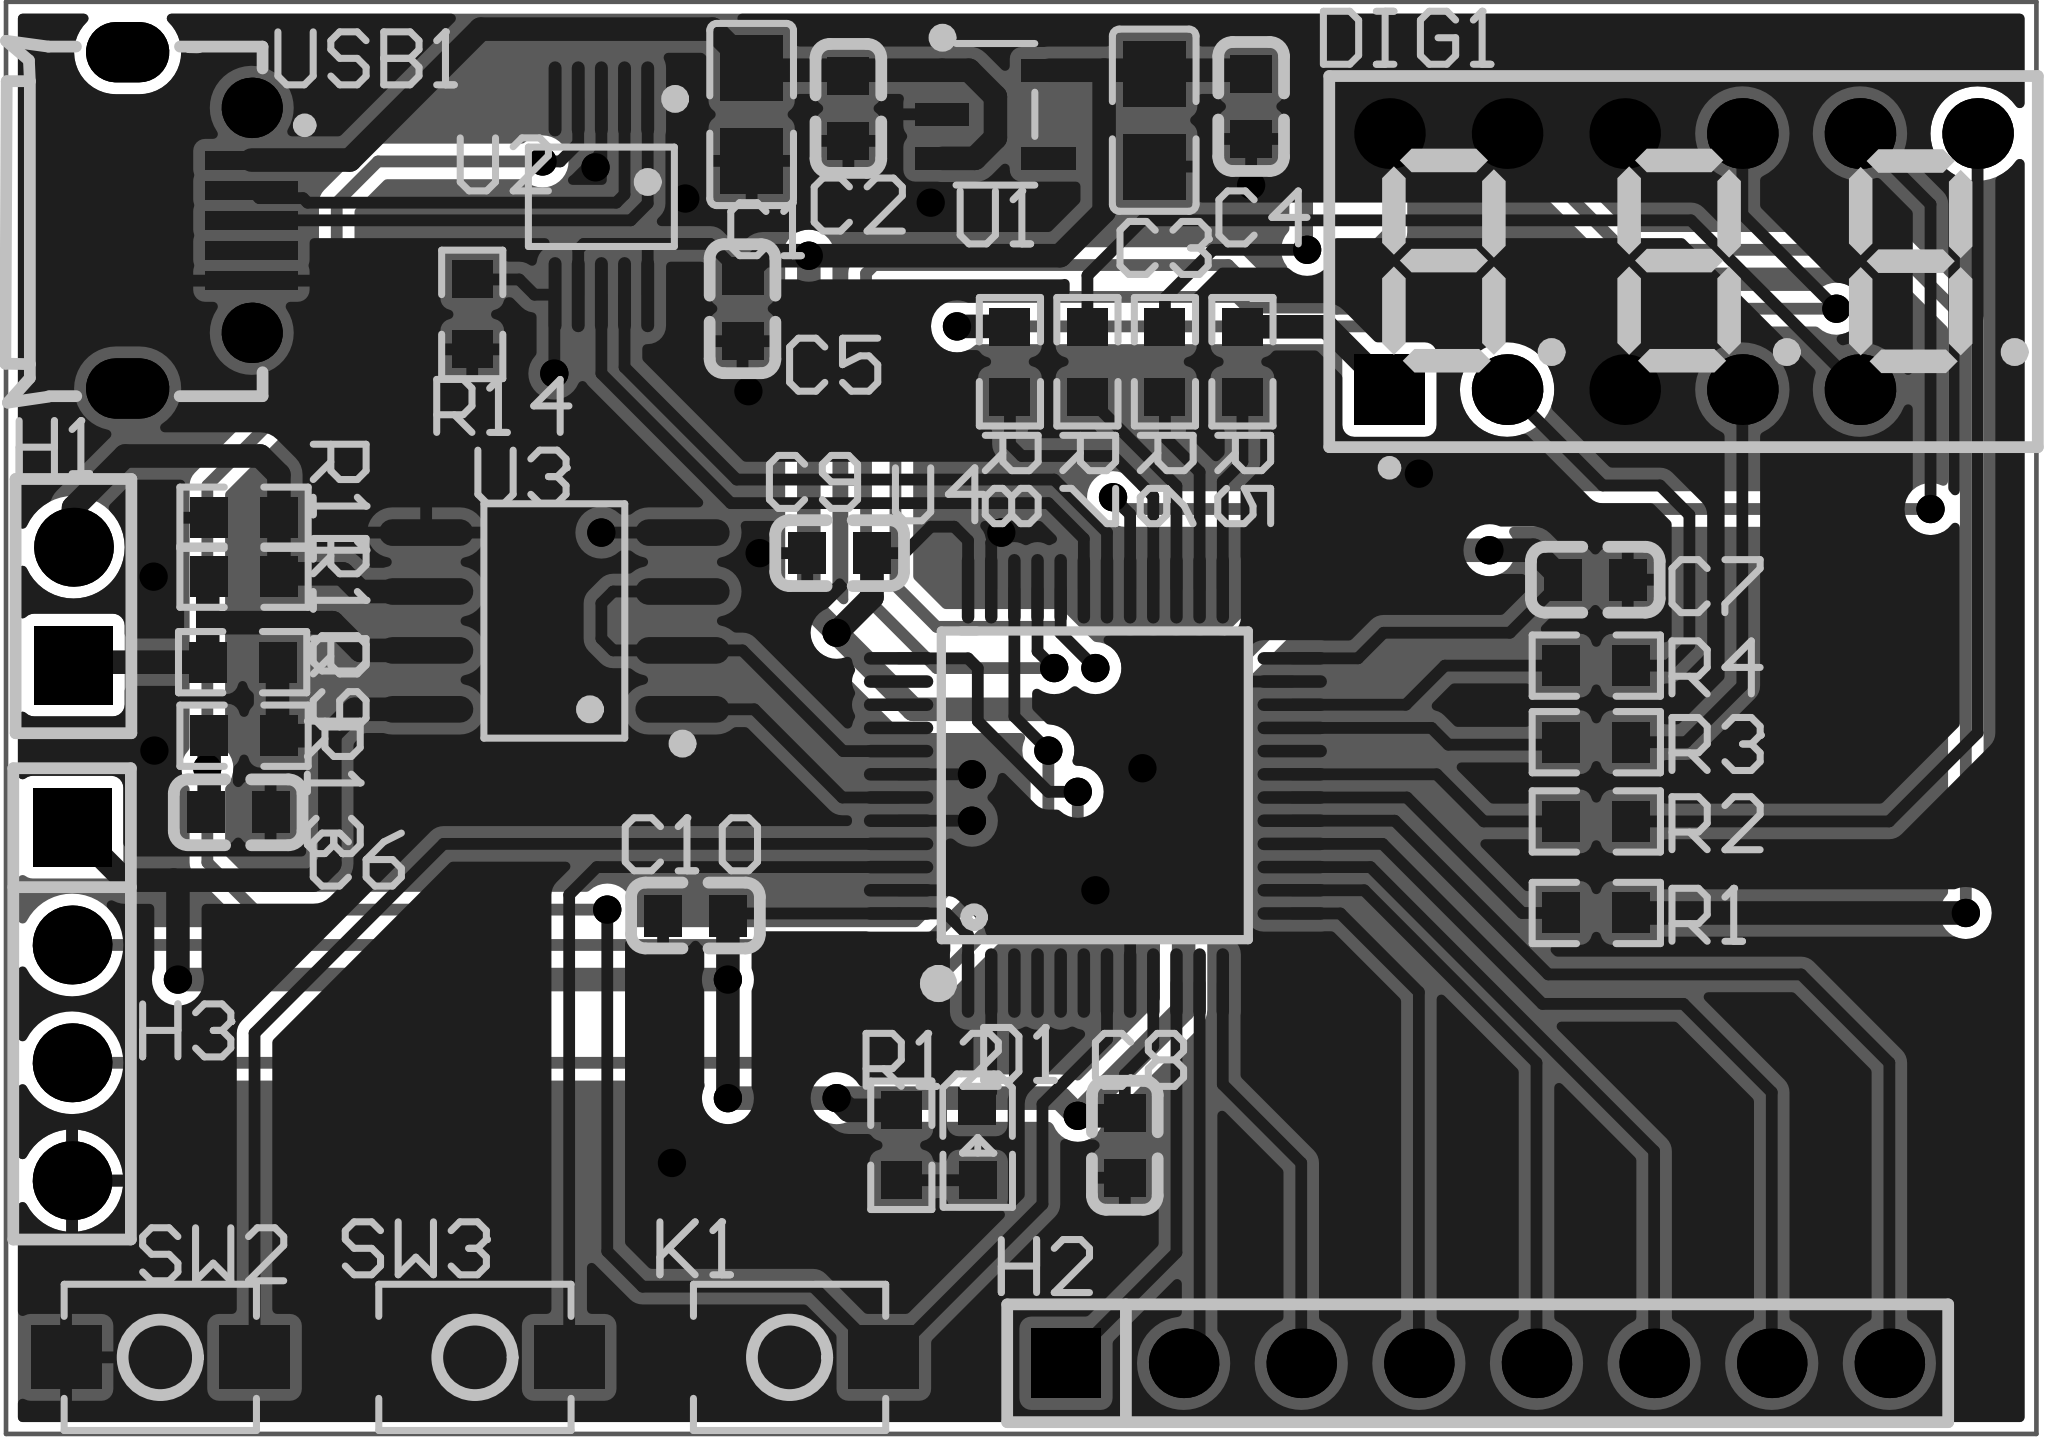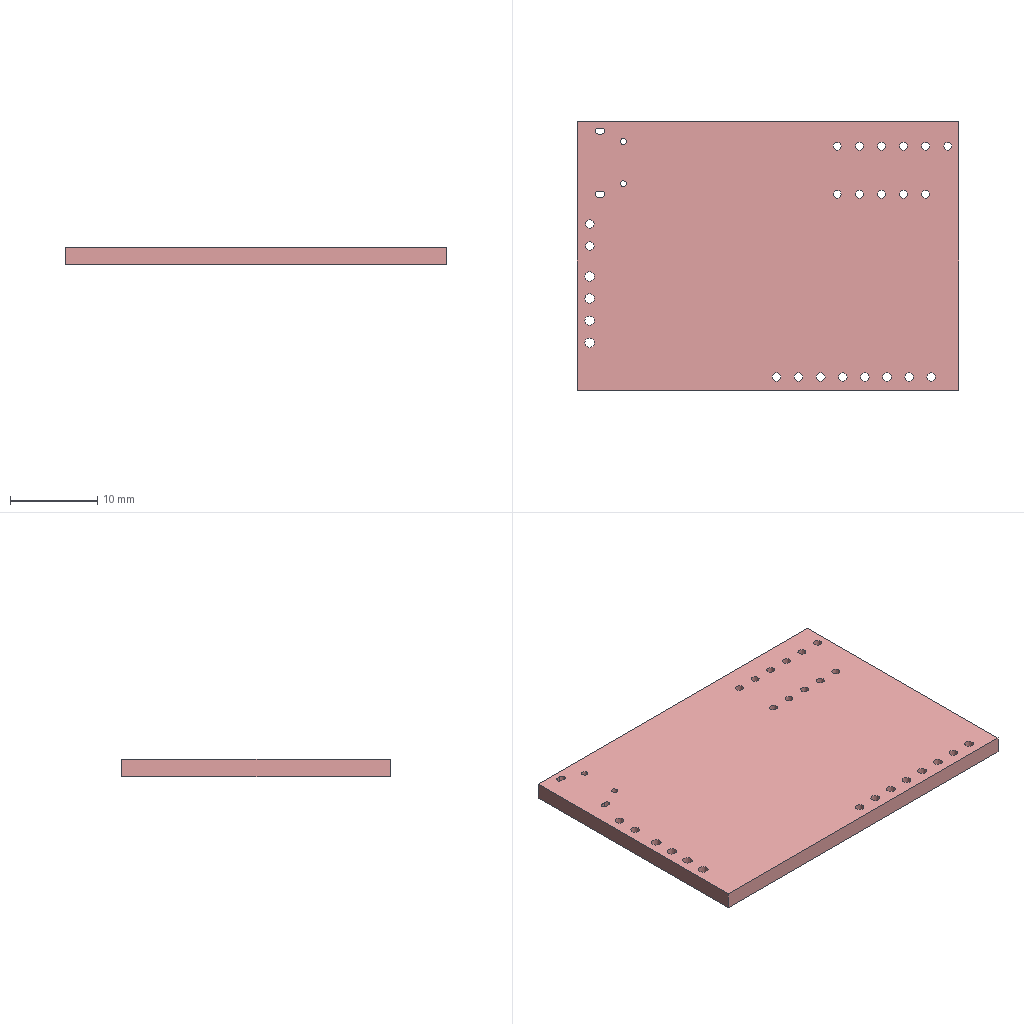Circuit board layout | Altium Designer | box 43.8 x 30.9 x 2 mm
Layer stack:
# Altium Designer layer stack of  (unit mm; dielectric type: 0 none, 1 core, 2 prepreg, 3 surface material)
index,name,kind,layer,copper_thickness_mm,dielectric_type,dielectric_thickness_mm,dielectric_material,dielectric_constant
0,Top Paste Mask Layer,other,,,,,,
1,Top Silkscreen Layer,other,,,,,,
2,Top Solder Mask Layer,dielectric,,,3,0.01,,3.3
3,Top Layer,copper,Top Layer,0.035,,,,
4,Dielectric1,dielectric,,,3,1.51,FR4,4.5
5,Mid-Layer 2,copper,Mid-Layer 2,0.0356,,,,
6,Dielectric2,dielectric,,,0,0.32,FR-4,4.8
7,Bottom Layer,copper,Bottom Layer,0.035,,,,
8,Bottom Solder Mask Layer,dielectric,,,3,0.01,,3.3
9,Bottom Silkscreen Layer,other,,,,,,
10,Bottom Paste Mask Layer,other,,,,,,
# drill layer pairs: low layer,high layer
drill_pair,Top Layer,Bottom Layer
Part placement:
Designator,Comment,Layer,Footprint,Center-X(mm),Center-Y(mm),Rotation
C1,475,TopLayer,C0805,96.266,107.692,90
C2,104,TopLayer,C0603,98.356,107.823,90
C3,335,TopLayer,C0805,104.96,107.569,90
C4,104,TopLayer,C0603,107.053,107.865,90
C5,104,TopLayer,C0603,96.07,103.505,90
C6,104,TopLayer,C0603,85.178,92.649,180
C7,104,TopLayer,C0603,114.485,97.663,180
C8,104,TopLayer,C0603,104.325,85.471,90
C9,104,TopLayer,C0603,98.167,98.236,0
C10,104,TopLayer,C0603,95.054,90.424,0
D1,,TopLayer,LED_0603,101.142,85.522,270
DIG1,FJ2352AH,TopLayer,LED-SEG-TH_FJ2352AH,116.39,104.521,0
H1,,TopLayer,HDR-TH_2P-P2.54-V-F,81.622,97.094,90
H2,B-2100S08P-A110,TopLayer,HDR-TH_8P-P2.54-V-M,111.945,80.772,0
H3,PZ254V-11-04P,TopLayer,HDR-TH_4P-P2.54-V-M,81.592,88.519,270
K1,HX 3x4x2-2P-2.5N,TopLayer,SW-SMD_L4.0-W2.9-LS5.0,97.086,80.899,0
R1,1K,TopLayer,R0603,114.506,90.478,180
R2,1K,TopLayer,R0603,114.506,92.452,180
R3,1K,TopLayer,R0603,114.506,94.16,180
R4,1K,TopLayer,R0603,114.506,95.811,180
R5,1K,TopLayer,R0603,106.865,102.362,270
R6,1K,TopLayer,R0603,105.191,102.362,270
R7,1K,TopLayer,R0603,103.517,102.362,270
R8,1K,TopLayer,R0603,101.844,102.362,270
R9,10K,TopLayer,R0603,85.275,95.885,180
R10,120,TopLayer,R0603,85.305,97.729,180
R11,10K,TopLayer,R0603,85.305,98.999,0
R12,1K,TopLayer,R0603,99.499,85.471,270
R13,10K,TopLayer,R0603,85.305,94.3,0
R14,4.7K,TopLayer,R0603,90.233,103.382,90
SW2,HX 3x4x2-2P-2.5N,TopLayer,SW-SMD_L4.0-W2.9-LS5.0,83.497,80.899,0
SW3,HX 3x4x2-2P-2.5N,TopLayer,SW-SMD_L4.0-W2.9-LS5.0,90.291,80.899,0
U1,ME6211C33M5G-N,TopLayer,SOT-23-5_L3.0-W1.7-P0.95-LS2.8-BL,101.531,107.696,270
U2,CH340X,TopLayer,MSOP-10_L3.0-W3.0-P0.50-LS5.0-BL,93.022,105.918,180
U3,SP3485EEN(UMW),TopLayer,SOP-8_L5.0-W4.0-P1.27-LS6.0-BL,92.006,96.774,90
U4,STM32F103C6T6ATR,TopLayer,LQFP-48_L7.0-W7.0-P0.50-LS9.0-BL,103.69,93.218,0
USB1,MicroXNJ,TopLayer,MICRO-USB-SMD_MICROXNJ_1,84.132,105.41,270
Pad and via stacks:
# Altium Designer via and pad stacks of  (unit mm). Each distinct definition once, with the count of objects using it.
# via: kind,start_layer,end_layer,hole_mm,diameter_mm,mode(0 simple;1 top-mid-bottom;2 full stack),diameter_per_layer,count,example_net
# pad: kind,layer,hole_mm,hole_type(0 round;1 square;2 slot),plating,top_size,top_shape(1 round;2 rect;3 octagon;9 rounded rect),mid_size,bottom_size,mode,footprint,size_per_layer,count,example
pad,Top Layer,0,0,plated,1.41x1.35,2,1.41x1.35,1.41x1.35,0,C0805,,4,C1.2
pad,Top Layer,0,0,plated,0.8x0.9,2,0.8x0.9,0.8x0.9,0,C0603,,16,C2.2
pad,Top Layer,0,0,plated,0.8001x0.8001,2,0.8001x0.8001,0.8001x0.8001,0,LED_0603,,2,D1.1
pad,Top Layer,0,0,plated,1.53x1.36,2,1.53x1.36,1.53x1.36,0,SW-SMD_L4.0-W2.9-LS5.0,,6,K1.1
pad,Top Layer,0,0,plated,0.8065x0.864,2,0.8065x0.864,0.8065x0.864,0,R0603,,28,R1.2
pad,Top Layer,0,0,plated,0.49x1.157,2,0.49x1.157,0.49x1.157,0,SOT-23-5_L3.0-W1.7-P0.95-LS2.8-BL,,3,U1.1
pad,Top Layer,0,0,plated,0.49x1.175,2,0.49x1.175,0.49x1.175,0,SOT-23-5_L3.0-W1.7-P0.95-LS2.8-BL,,2,U1.4
pad,Top Layer,0,0,plated,0.28x1.62,1,0.28x1.62,0.28x1.62,0,MSOP-10_L3.0-W3.0-P0.50-LS5.0-BL,,10,U2.1
pad,Top Layer,0,0,plated,0.574x2.035,1,0.574x2.035,0.574x2.035,0,SOP-8_L5.0-W4.0-P1.27-LS6.0-BL,,8,U3.1
pad,Top Layer,0,0,plated,0.27x1.5,1,0.27x1.5,0.27x1.5,0,LQFP-48_L7.0-W7.0-P0.50-LS9.0-BL,,24,U4.1
pad,Top Layer,0,0,plated,1.5x0.27,1,1.5x0.27,1.5x0.27,0,LQFP-48_L7.0-W7.0-P0.50-LS9.0-BL,,24,U4.13
pad,Top Layer,0,0,plated,0.4x2,2,0.4x2,0.4x2,0,MICRO-USB-SMD_MICROXNJ_1,,5,USB1.5
pad,Multi-Layer,0.9144,0,plated,1.524x1.524,2,1.524x1.524,1.524x1.524,0,LED-SEG-TH_FJ2352AH,,1,DIG1.1
pad,Multi-Layer,0.9144,0,plated,1.524x1.524,1,1.524x1.524,1.524x1.524,0,LED-SEG-TH_FJ2352AH,,10,DIG1.2
pad,Multi-Layer,1,0,plated,1.7x1.7,2,1.7x1.7,1.7x1.7,0,HDR-TH_2P-P2.54-V-F,,1,H1.1
pad,Multi-Layer,1,0,plated,1.7x1.7,1,1.7x1.7,1.7x1.7,0,HDR-TH_2P-P2.54-V-F,,1,H1.2
pad,Multi-Layer,1,0,plated,1.5x1.5,2,1.5x1.5,1.5x1.5,0,HDR-TH_8P-P2.54-V-M,,1,H2.1
pad,Multi-Layer,1,0,plated,1.5x1.5,1,1.5x1.5,1.5x1.5,0,HDR-TH_8P-P2.54-V-M,,7,H2.2
pad,Multi-Layer,1.1,0,plated,1.7x1.7,2,1.7x1.7,1.7x1.7,0,HDR-TH_4P-P2.54-V-M,,1,H3.1
pad,Multi-Layer,1.1,0,plated,1.7x1.7,1,1.7x1.7,1.7x1.7,0,HDR-TH_4P-P2.54-V-M,,3,H3.2
pad,Multi-Layer,0.7,0,plated,1.3x1.3,1,1.3x1.3,1.3x1.3,0,MICRO-USB-SMD_MICROXNJ_1,,2,USB1.6
pad,Multi-Layer,0.7,2,plated,1.3x1.8,1,1.3x1.8,1.3x1.8,0,MICRO-USB-SMD_MICROXNJ_1,,2,USB1.8
via,Top Layer,Bottom Layer,0.3048,0.61,0,,38,A
Copper pours:
name,layer,net,type(0 solid;1 hatched;2 none)
Bottom Layer-GND,Bottom Layer,GND,0
Top Layer-GND,Top Layer,GND,0